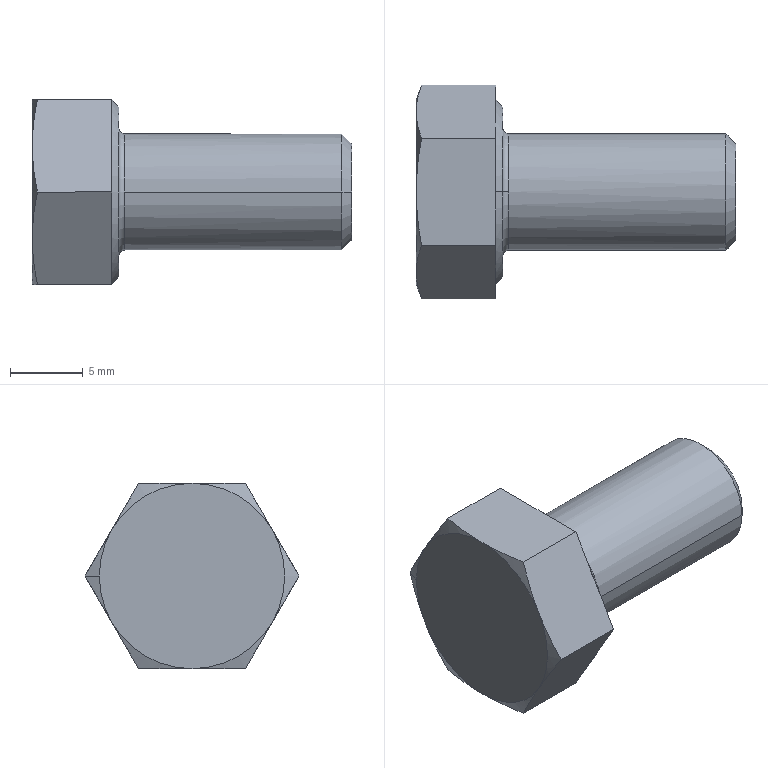Part | NX | features BREP 1 | 1 solid | 30 faces | box 21.95 x 14.699 x 12.73 mm | volume 1621 mm3 | plane 15 | cone 11 | torus 2 | cylinder 2 | commonest cylinder face diameters 8 x2
STEP:
#1=CARTESIAN_POINT('',(5.45,0.,-6.365));
#2=VERTEX_POINT('',#1);
#3=CARTESIAN_POINT('',(5.95,0.,-5.815));
#4=VERTEX_POINT('',#3);
#5=CARTESIAN_POINT('',(5.95,0.,-5.815));
#6=DIRECTION('',(-0.6727,0.,-0.7399));
#7=VECTOR('',#6,1000.);
#8=LINE('',#5,#7);
#9=EDGE_CURVE('',#2,#4,#8,.F.);
#10=ORIENTED_EDGE('',*,*,#9,.T.);
#11=CARTESIAN_POINT('',(5.95,0.,5.815));
#12=VERTEX_POINT('',#11);
#13=CARTESIAN_POINT('',(5.95,0.,0.));
#14=DIRECTION('',(-1.,0.,0.));
#15=DIRECTION('',(0.,0.,1.));
#16=AXIS2_PLACEMENT_3D('',#13,#14,#15);
#17=CIRCLE('',#16,5.815);
#18=EDGE_CURVE('',#4,#12,#17,.T.);
#19=ORIENTED_EDGE('',*,*,#18,.T.);
#20=CARTESIAN_POINT('',(5.45,0.,6.365));
#21=VERTEX_POINT('',#20);
#22=CARTESIAN_POINT('',(5.95,0.,5.815));
#23=DIRECTION('',(-0.6727,0.,0.7399));
#24=VECTOR('',#23,1000.);
#25=LINE('',#22,#24);
#26=EDGE_CURVE('',#21,#12,#25,.F.);
#27=ORIENTED_EDGE('',*,*,#26,.F.);
#28=CARTESIAN_POINT('',(5.45,-5.512,3.183));
#29=VERTEX_POINT('',#28);
#30=CARTESIAN_POINT('',(5.45,0.,0.));
#31=DIRECTION('',(-1.,0.,0.));
#32=DIRECTION('',(0.,0.,1.));
#33=AXIS2_PLACEMENT_3D('',#30,#31,#32);
#34=CIRCLE('',#33,6.365);
#35=EDGE_CURVE('',#29,#21,#34,.T.);
#36=ORIENTED_EDGE('',*,*,#35,.F.);
#37=CARTESIAN_POINT('',(5.45,-5.512,-3.183));
#38=VERTEX_POINT('',#37);
#39=CARTESIAN_POINT('',(5.45,0.,0.));
#40=DIRECTION('',(-1.,0.,0.));
#41=DIRECTION('',(0.,0.,1.));
#42=AXIS2_PLACEMENT_3D('',#39,#40,#41);
#43=CIRCLE('',#42,6.365);
#44=EDGE_CURVE('',#38,#29,#43,.T.);
#45=ORIENTED_EDGE('',*,*,#44,.F.);
#46=CARTESIAN_POINT('',(5.45,0.,0.));
#47=DIRECTION('',(-1.,0.,0.));
#48=DIRECTION('',(0.,0.,1.));
#49=AXIS2_PLACEMENT_3D('',#46,#47,#48);
#50=CIRCLE('',#49,6.365);
#51=EDGE_CURVE('',#2,#38,#50,.T.);
#52=ORIENTED_EDGE('',*,*,#51,.F.);
#53=EDGE_LOOP('',(#10,#19,#27,#36,#45,#52));
#54=FACE_BOUND('',#53,.T.);
#55=CARTESIAN_POINT('',(5.95,0.,0.));
#56=DIRECTION('',(-1.,0.,0.));
#57=DIRECTION('',(0.,0.,-1.));
#58=AXIS2_PLACEMENT_3D('',#55,#56,#57);
#59=CONICAL_SURFACE('',#58,5.815,0.833);
#60=ADVANCED_FACE('',(#54),#59,.T.);
#61=CARTESIAN_POINT('',(5.95,0.,4.4));
#62=VERTEX_POINT('',#61);
#63=CARTESIAN_POINT('',(5.95,0.,-4.4));
#64=VERTEX_POINT('',#63);
#65=CARTESIAN_POINT('',(5.95,0.,0.));
#66=DIRECTION('',(-1.,0.,0.));
#67=DIRECTION('',(0.,0.,1.));
#68=AXIS2_PLACEMENT_3D('',#65,#66,#67);
#69=CIRCLE('',#68,4.4);
#70=EDGE_CURVE('',#62,#64,#69,.T.);
#71=ORIENTED_EDGE('',*,*,#70,.T.);
#72=CARTESIAN_POINT('',(5.95,0.,0.));
#73=DIRECTION('',(-1.,0.,0.));
#74=DIRECTION('',(0.,0.,1.));
#75=AXIS2_PLACEMENT_3D('',#72,#73,#74);
#76=CIRCLE('',#75,4.4);
#77=EDGE_CURVE('',#64,#62,#76,.T.);
#78=ORIENTED_EDGE('',*,*,#77,.T.);
#79=EDGE_LOOP('',(#71,#78));
#80=FACE_BOUND('',#79,.T.);
#81=CARTESIAN_POINT('',(5.95,0.,0.));
#82=DIRECTION('',(-1.,0.,0.));
#83=DIRECTION('',(0.,0.,1.));
#84=AXIS2_PLACEMENT_3D('',#81,#82,#83);
#85=CIRCLE('',#84,5.815);
#86=EDGE_CURVE('',#12,#4,#85,.T.);
#87=ORIENTED_EDGE('',*,*,#86,.F.);
#88=ORIENTED_EDGE('',*,*,#18,.F.);
#89=EDGE_LOOP('',(#87,#88));
#90=FACE_BOUND('',#89,.T.);
#91=CARTESIAN_POINT('',(5.95,0.,0.));
#92=DIRECTION('',(-1.,0.,0.));
#93=DIRECTION('',(0.,0.,-1.));
#94=AXIS2_PLACEMENT_3D('',#91,#92,#93);
#95=PLANE('',#94);
#96=ADVANCED_FACE('',(#80,#90),#95,.F.);
#97=CARTESIAN_POINT('',(5.45,-3.675,6.365));
#98=VERTEX_POINT('',#97);
#99=CARTESIAN_POINT('',(5.45,-3.675,6.365));
#100=DIRECTION('',(0.,-0.5,-0.866));
#101=VECTOR('',#100,1000.);
#102=LINE('',#99,#101);
#103=EDGE_CURVE('',#98,#29,#102,.T.);
#104=ORIENTED_EDGE('',*,*,#103,.T.);
#105=ORIENTED_EDGE('',*,*,#35,.T.);
#106=CARTESIAN_POINT('',(5.45,3.675,6.365));
#107=DIRECTION('',(0.,-1.,0.));
#108=VECTOR('',#107,1000.);
#109=LINE('',#106,#108);
#110=EDGE_CURVE('',#21,#98,#109,.T.);
#111=ORIENTED_EDGE('',*,*,#110,.T.);
#112=EDGE_LOOP('',(#104,#105,#111));
#113=FACE_BOUND('',#112,.T.);
#114=CARTESIAN_POINT('',(5.45,0.,12.73));
#115=DIRECTION('',(-1.,0.,0.));
#116=DIRECTION('',(0.,0.,-1.));
#117=AXIS2_PLACEMENT_3D('',#114,#115,#116);
#118=PLANE('',#117);
#119=ADVANCED_FACE('',(#113),#118,.F.);
#120=ORIENTED_EDGE('',*,*,#86,.T.);
#121=ORIENTED_EDGE('',*,*,#9,.F.);
#122=CARTESIAN_POINT('',(5.45,5.512,-3.183));
#123=VERTEX_POINT('',#122);
#124=CARTESIAN_POINT('',(5.45,0.,0.));
#125=DIRECTION('',(-1.,0.,0.));
#126=DIRECTION('',(0.,0.,1.));
#127=AXIS2_PLACEMENT_3D('',#124,#125,#126);
#128=CIRCLE('',#127,6.365);
#129=EDGE_CURVE('',#123,#2,#128,.T.);
#130=ORIENTED_EDGE('',*,*,#129,.F.);
#131=CARTESIAN_POINT('',(5.45,5.512,3.183));
#132=VERTEX_POINT('',#131);
#133=CARTESIAN_POINT('',(5.45,0.,0.));
#134=DIRECTION('',(-1.,0.,0.));
#135=DIRECTION('',(0.,0.,1.));
#136=AXIS2_PLACEMENT_3D('',#133,#134,#135);
#137=CIRCLE('',#136,6.365);
#138=EDGE_CURVE('',#132,#123,#137,.T.);
#139=ORIENTED_EDGE('',*,*,#138,.F.);
#140=CARTESIAN_POINT('',(5.45,0.,0.));
#141=DIRECTION('',(-1.,0.,0.));
#142=DIRECTION('',(0.,0.,1.));
#143=AXIS2_PLACEMENT_3D('',#140,#141,#142);
#144=CIRCLE('',#143,6.365);
#145=EDGE_CURVE('',#21,#132,#144,.T.);
#146=ORIENTED_EDGE('',*,*,#145,.F.);
#147=ORIENTED_EDGE('',*,*,#26,.T.);
#148=EDGE_LOOP('',(#120,#121,#130,#139,#146,#147));
#149=FACE_BOUND('',#148,.T.);
#150=CARTESIAN_POINT('',(5.95,0.,0.));
#151=DIRECTION('',(-1.,0.,0.));
#152=DIRECTION('',(0.,0.,-1.));
#153=AXIS2_PLACEMENT_3D('',#150,#151,#152);
#154=CONICAL_SURFACE('',#153,5.815,0.833);
#155=ADVANCED_FACE('',(#149),#154,.T.);
#156=CARTESIAN_POINT('',(5.45,-3.675,-6.365));
#157=VERTEX_POINT('',#156);
#158=CARTESIAN_POINT('',(5.45,-3.675,-6.365));
#159=DIRECTION('',(0.,1.,0.));
#160=VECTOR('',#159,1000.);
#161=LINE('',#158,#160);
#162=EDGE_CURVE('',#157,#2,#161,.T.);
#163=ORIENTED_EDGE('',*,*,#162,.T.);
#164=ORIENTED_EDGE('',*,*,#51,.T.);
#165=CARTESIAN_POINT('',(5.45,-7.35,0.));
#166=DIRECTION('',(0.,0.5,-0.866));
#167=VECTOR('',#166,1000.);
#168=LINE('',#165,#167);
#169=EDGE_CURVE('',#38,#157,#168,.T.);
#170=ORIENTED_EDGE('',*,*,#169,.T.);
#171=EDGE_LOOP('',(#163,#164,#170));
#172=FACE_BOUND('',#171,.T.);
#173=CARTESIAN_POINT('',(5.45,0.,12.73));
#174=DIRECTION('',(-1.,0.,0.));
#175=DIRECTION('',(0.,0.,-1.));
#176=AXIS2_PLACEMENT_3D('',#173,#174,#175);
#177=PLANE('',#176);
#178=ADVANCED_FACE('',(#172),#177,.F.);
#179=CARTESIAN_POINT('',(5.45,-7.35,0.));
#180=VERTEX_POINT('',#179);
#181=CARTESIAN_POINT('',(5.45,-7.35,0.));
#182=DIRECTION('',(0.,0.5,-0.866));
#183=VECTOR('',#182,1000.);
#184=LINE('',#181,#183);
#185=EDGE_CURVE('',#180,#38,#184,.T.);
#186=ORIENTED_EDGE('',*,*,#185,.T.);
#187=ORIENTED_EDGE('',*,*,#44,.T.);
#188=CARTESIAN_POINT('',(5.45,-3.675,6.365));
#189=DIRECTION('',(0.,-0.5,-0.866));
#190=VECTOR('',#189,1000.);
#191=LINE('',#188,#190);
#192=EDGE_CURVE('',#29,#180,#191,.T.);
#193=ORIENTED_EDGE('',*,*,#192,.T.);
#194=EDGE_LOOP('',(#186,#187,#193));
#195=FACE_BOUND('',#194,.T.);
#196=CARTESIAN_POINT('',(5.45,0.,12.73));
#197=DIRECTION('',(-1.,0.,0.));
#198=DIRECTION('',(0.,0.,-1.));
#199=AXIS2_PLACEMENT_3D('',#196,#197,#198);
#200=PLANE('',#199);
#201=ADVANCED_FACE('',(#195),#200,.F.);
#202=ORIENTED_EDGE('',*,*,#77,.F.);
#203=CARTESIAN_POINT('',(6.35,0.,-4.));
#204=VERTEX_POINT('',#203);
#205=CARTESIAN_POINT('',(6.35,0.,-4.4));
#206=DIRECTION('',(0.,1.,0.));
#207=DIRECTION('',(0.,0.,1.));
#208=AXIS2_PLACEMENT_3D('',#205,#206,#207);
#209=CIRCLE('',#208,0.4);
#210=EDGE_CURVE('',#64,#204,#209,.T.);
#211=ORIENTED_EDGE('',*,*,#210,.T.);
#212=CARTESIAN_POINT('',(6.35,-4.,0.));
#213=VERTEX_POINT('',#212);
#214=CARTESIAN_POINT('',(6.35,0.,0.));
#215=DIRECTION('',(1.,0.,0.));
#216=DIRECTION('',(0.,0.,1.));
#217=AXIS2_PLACEMENT_3D('',#214,#215,#216);
#218=CIRCLE('',#217,4.);
#219=EDGE_CURVE('',#213,#204,#218,.T.);
#220=ORIENTED_EDGE('',*,*,#219,.F.);
#221=CARTESIAN_POINT('',(6.35,0.,4.));
#222=VERTEX_POINT('',#221);
#223=CARTESIAN_POINT('',(6.35,0.,0.));
#224=DIRECTION('',(1.,0.,0.));
#225=DIRECTION('',(0.,0.,1.));
#226=AXIS2_PLACEMENT_3D('',#223,#224,#225);
#227=CIRCLE('',#226,4.);
#228=EDGE_CURVE('',#222,#213,#227,.T.);
#229=ORIENTED_EDGE('',*,*,#228,.F.);
#230=CARTESIAN_POINT('',(6.35,0.,4.4));
#231=DIRECTION('',(0.,-1.,0.));
#232=DIRECTION('',(0.,0.,-1.));
#233=AXIS2_PLACEMENT_3D('',#230,#231,#232);
#234=CIRCLE('',#233,0.4);
#235=EDGE_CURVE('',#62,#222,#234,.T.);
#236=ORIENTED_EDGE('',*,*,#235,.F.);
#237=EDGE_LOOP('',(#202,#211,#220,#229,#236));
#238=FACE_BOUND('',#237,.T.);
#239=CARTESIAN_POINT('',(6.35,0.,0.));
#240=DIRECTION('',(-1.,0.,0.));
#241=DIRECTION('',(0.,0.,-1.));
#242=AXIS2_PLACEMENT_3D('',#239,#240,#241);
#243=TOROIDAL_SURFACE('',#242,4.4,0.4);
#244=ADVANCED_FACE('',(#238),#243,.F.);
#245=ORIENTED_EDGE('',*,*,#210,.F.);
#246=ORIENTED_EDGE('',*,*,#70,.F.);
#247=ORIENTED_EDGE('',*,*,#235,.T.);
#248=CARTESIAN_POINT('',(6.35,4.,0.));
#249=VERTEX_POINT('',#248);
#250=CARTESIAN_POINT('',(6.35,0.,0.));
#251=DIRECTION('',(1.,0.,0.));
#252=DIRECTION('',(0.,0.,1.));
#253=AXIS2_PLACEMENT_3D('',#250,#251,#252);
#254=CIRCLE('',#253,4.);
#255=EDGE_CURVE('',#249,#222,#254,.T.);
#256=ORIENTED_EDGE('',*,*,#255,.F.);
#257=CARTESIAN_POINT('',(6.35,0.,0.));
#258=DIRECTION('',(1.,0.,0.));
#259=DIRECTION('',(0.,0.,1.));
#260=AXIS2_PLACEMENT_3D('',#257,#258,#259);
#261=CIRCLE('',#260,4.);
#262=EDGE_CURVE('',#204,#249,#261,.T.);
#263=ORIENTED_EDGE('',*,*,#262,.F.);
#264=EDGE_LOOP('',(#245,#246,#247,#256,#263));
#265=FACE_BOUND('',#264,.T.);
#266=CARTESIAN_POINT('',(6.35,0.,0.));
#267=DIRECTION('',(-1.,0.,0.));
#268=DIRECTION('',(0.,0.,-1.));
#269=AXIS2_PLACEMENT_3D('',#266,#267,#268);
#270=TOROIDAL_SURFACE('',#269,4.4,0.4);
#271=ADVANCED_FACE('',(#265),#270,.F.);
#272=CARTESIAN_POINT('',(0.3584,-3.675,6.365));
#273=VERTEX_POINT('',#272);
#274=CARTESIAN_POINT('',(0.,0.,6.365));
#275=VERTEX_POINT('',#274);
#276=CARTESIAN_POINT('',(0.3584,-3.675,6.365));
#277=CARTESIAN_POINT('',(0.1373,-2.46,6.365));
#278=CARTESIAN_POINT('',(0.,-1.237,6.365));
#279=CARTESIAN_POINT('',(0.,0.,6.365));
#280=B_SPLINE_CURVE_WITH_KNOTS('',3,(#276,#277,#278,#279),.UNSPECIFIED.,.F.,.F.,(4,4),(0.,0.003692),.UNSPECIFIED.);
#281=EDGE_CURVE('',#273,#275,#280,.T.);
#282=ORIENTED_EDGE('',*,*,#281,.F.);
#283=CARTESIAN_POINT('',(5.45,-3.675,6.365));
#284=DIRECTION('',(-1.,0.,0.));
#285=VECTOR('',#284,1000.);
#286=LINE('',#283,#285);
#287=EDGE_CURVE('',#98,#273,#286,.T.);
#288=ORIENTED_EDGE('',*,*,#287,.F.);
#289=ORIENTED_EDGE('',*,*,#110,.F.);
#290=CARTESIAN_POINT('',(5.45,3.675,6.365));
#291=VERTEX_POINT('',#290);
#292=CARTESIAN_POINT('',(5.45,3.675,6.365));
#293=DIRECTION('',(0.,-1.,0.));
#294=VECTOR('',#293,1000.);
#295=LINE('',#292,#294);
#296=EDGE_CURVE('',#291,#21,#295,.T.);
#297=ORIENTED_EDGE('',*,*,#296,.F.);
#298=CARTESIAN_POINT('',(0.3584,3.675,6.365));
#299=VERTEX_POINT('',#298);
#300=CARTESIAN_POINT('',(5.45,3.675,6.365));
#301=DIRECTION('',(-1.,0.,0.));
#302=VECTOR('',#301,1000.);
#303=LINE('',#300,#302);
#304=EDGE_CURVE('',#291,#299,#303,.T.);
#305=ORIENTED_EDGE('',*,*,#304,.T.);
#306=CARTESIAN_POINT('',(0.,0.,6.365));
#307=CARTESIAN_POINT('',(0.,1.237,6.365));
#308=CARTESIAN_POINT('',(0.1373,2.46,6.365));
#309=CARTESIAN_POINT('',(0.3584,3.675,6.365));
#310=B_SPLINE_CURVE_WITH_KNOTS('',3,(#306,#307,#308,#309),.UNSPECIFIED.,.F.,.F.,(4,4),(0.,0.003692),.UNSPECIFIED.);
#311=EDGE_CURVE('',#275,#299,#310,.T.);
#312=ORIENTED_EDGE('',*,*,#311,.F.);
#313=EDGE_LOOP('',(#282,#288,#289,#297,#305,#312));
#314=FACE_BOUND('',#313,.T.);
#315=CARTESIAN_POINT('',(5.45,3.675,6.365));
#316=DIRECTION('',(0.,0.,-1.));
#317=DIRECTION('',(1.,0.,0.));
#318=AXIS2_PLACEMENT_3D('',#315,#316,#317);
#319=PLANE('',#318);
#320=ADVANCED_FACE('',(#314),#319,.F.);
#321=CARTESIAN_POINT('',(0.3584,-7.35,0.));
#322=VERTEX_POINT('',#321);
#323=CARTESIAN_POINT('',(0.,-5.512,3.183));
#324=VERTEX_POINT('',#323);
#325=CARTESIAN_POINT('',(0.3584,-7.35,0.));
#326=CARTESIAN_POINT('',(0.1373,-6.742,1.052));
#327=CARTESIAN_POINT('',(0.,-6.131,2.112));
#328=CARTESIAN_POINT('',(0.,-5.512,3.183));
#329=B_SPLINE_CURVE_WITH_KNOTS('',3,(#325,#326,#327,#328),.UNSPECIFIED.,.F.,.F.,(4,4),(0.,0.003692),.UNSPECIFIED.);
#330=EDGE_CURVE('',#322,#324,#329,.T.);
#331=ORIENTED_EDGE('',*,*,#330,.F.);
#332=CARTESIAN_POINT('',(5.45,-7.35,0.));
#333=DIRECTION('',(-1.,0.,0.));
#334=VECTOR('',#333,1000.);
#335=LINE('',#332,#334);
#336=EDGE_CURVE('',#180,#322,#335,.T.);
#337=ORIENTED_EDGE('',*,*,#336,.F.);
#338=ORIENTED_EDGE('',*,*,#192,.F.);
#339=ORIENTED_EDGE('',*,*,#103,.F.);
#340=ORIENTED_EDGE('',*,*,#287,.T.);
#341=CARTESIAN_POINT('',(0.,-5.512,3.183));
#342=CARTESIAN_POINT('',(0.,-4.894,4.253));
#343=CARTESIAN_POINT('',(0.1373,-4.282,5.313));
#344=CARTESIAN_POINT('',(0.3584,-3.675,6.365));
#345=B_SPLINE_CURVE_WITH_KNOTS('',3,(#341,#342,#343,#344),.UNSPECIFIED.,.F.,.F.,(4,4),(0.,0.003692),.UNSPECIFIED.);
#346=EDGE_CURVE('',#324,#273,#345,.T.);
#347=ORIENTED_EDGE('',*,*,#346,.F.);
#348=EDGE_LOOP('',(#331,#337,#338,#339,#340,#347));
#349=FACE_BOUND('',#348,.T.);
#350=CARTESIAN_POINT('',(5.45,-3.675,6.365));
#351=DIRECTION('',(0.,0.866,-0.5));
#352=DIRECTION('',(0.,-0.5,-0.866));
#353=AXIS2_PLACEMENT_3D('',#350,#351,#352);
#354=PLANE('',#353);
#355=ADVANCED_FACE('',(#349),#354,.F.);
#356=CARTESIAN_POINT('',(5.45,7.35,0.));
#357=VERTEX_POINT('',#356);
#358=CARTESIAN_POINT('',(5.45,7.35,0.));
#359=DIRECTION('',(0.,-0.5,0.866));
#360=VECTOR('',#359,1000.);
#361=LINE('',#358,#360);
#362=EDGE_CURVE('',#357,#132,#361,.T.);
#363=ORIENTED_EDGE('',*,*,#362,.T.);
#364=ORIENTED_EDGE('',*,*,#138,.T.);
#365=CARTESIAN_POINT('',(5.45,3.675,-6.365));
#366=DIRECTION('',(0.,0.5,0.866));
#367=VECTOR('',#366,1000.);
#368=LINE('',#365,#367);
#369=EDGE_CURVE('',#123,#357,#368,.T.);
#370=ORIENTED_EDGE('',*,*,#369,.T.);
#371=EDGE_LOOP('',(#363,#364,#370));
#372=FACE_BOUND('',#371,.T.);
#373=CARTESIAN_POINT('',(5.45,0.,12.73));
#374=DIRECTION('',(-1.,0.,0.));
#375=DIRECTION('',(0.,0.,-1.));
#376=AXIS2_PLACEMENT_3D('',#373,#374,#375);
#377=PLANE('',#376);
#378=ADVANCED_FACE('',(#372),#377,.F.);
#379=CARTESIAN_POINT('',(5.45,3.675,-6.365));
#380=VERTEX_POINT('',#379);
#381=CARTESIAN_POINT('',(5.45,3.675,-6.365));
#382=DIRECTION('',(0.,0.5,0.866));
#383=VECTOR('',#382,1000.);
#384=LINE('',#381,#383);
#385=EDGE_CURVE('',#380,#123,#384,.T.);
#386=ORIENTED_EDGE('',*,*,#385,.T.);
#387=ORIENTED_EDGE('',*,*,#129,.T.);
#388=CARTESIAN_POINT('',(5.45,-3.675,-6.365));
#389=DIRECTION('',(0.,1.,0.));
#390=VECTOR('',#389,1000.);
#391=LINE('',#388,#390);
#392=EDGE_CURVE('',#2,#380,#391,.T.);
#393=ORIENTED_EDGE('',*,*,#392,.T.);
#394=EDGE_LOOP('',(#386,#387,#393));
#395=FACE_BOUND('',#394,.T.);
#396=CARTESIAN_POINT('',(5.45,0.,12.73));
#397=DIRECTION('',(-1.,0.,0.));
#398=DIRECTION('',(0.,0.,-1.));
#399=AXIS2_PLACEMENT_3D('',#396,#397,#398);
#400=PLANE('',#399);
#401=ADVANCED_FACE('',(#395),#400,.F.);
#402=ORIENTED_EDGE('',*,*,#296,.T.);
#403=ORIENTED_EDGE('',*,*,#145,.T.);
#404=CARTESIAN_POINT('',(5.45,7.35,0.));
#405=DIRECTION('',(0.,-0.5,0.866));
#406=VECTOR('',#405,1000.);
#407=LINE('',#404,#406);
#408=EDGE_CURVE('',#132,#291,#407,.T.);
#409=ORIENTED_EDGE('',*,*,#408,.T.);
#410=EDGE_LOOP('',(#402,#403,#409));
#411=FACE_BOUND('',#410,.T.);
#412=CARTESIAN_POINT('',(5.45,0.,12.73));
#413=DIRECTION('',(-1.,0.,0.));
#414=DIRECTION('',(0.,0.,-1.));
#415=AXIS2_PLACEMENT_3D('',#412,#413,#414);
#416=PLANE('',#415);
#417=ADVANCED_FACE('',(#411),#416,.F.);
#418=CARTESIAN_POINT('',(0.3584,3.675,-6.365));
#419=VERTEX_POINT('',#418);
#420=CARTESIAN_POINT('',(0.,0.,-6.365));
#421=VERTEX_POINT('',#420);
#422=CARTESIAN_POINT('',(0.3584,3.675,-6.365));
#423=CARTESIAN_POINT('',(0.1373,2.46,-6.365));
#424=CARTESIAN_POINT('',(0.,1.237,-6.365));
#425=CARTESIAN_POINT('',(0.,0.,-6.365));
#426=B_SPLINE_CURVE_WITH_KNOTS('',3,(#422,#423,#424,#425),.UNSPECIFIED.,.F.,.F.,(4,4),(0.,0.003692),.UNSPECIFIED.);
#427=EDGE_CURVE('',#419,#421,#426,.T.);
#428=ORIENTED_EDGE('',*,*,#427,.F.);
#429=CARTESIAN_POINT('',(5.45,3.675,-6.365));
#430=DIRECTION('',(-1.,0.,0.));
#431=VECTOR('',#430,1000.);
#432=LINE('',#429,#431);
#433=EDGE_CURVE('',#380,#419,#432,.T.);
#434=ORIENTED_EDGE('',*,*,#433,.F.);
#435=ORIENTED_EDGE('',*,*,#392,.F.);
#436=ORIENTED_EDGE('',*,*,#162,.F.);
#437=CARTESIAN_POINT('',(0.3584,-3.675,-6.365));
#438=VERTEX_POINT('',#437);
#439=CARTESIAN_POINT('',(5.45,-3.675,-6.365));
#440=DIRECTION('',(-1.,0.,0.));
#441=VECTOR('',#440,1000.);
#442=LINE('',#439,#441);
#443=EDGE_CURVE('',#157,#438,#442,.T.);
#444=ORIENTED_EDGE('',*,*,#443,.T.);
#445=CARTESIAN_POINT('',(0.,0.,-6.365));
#446=CARTESIAN_POINT('',(0.,-1.237,-6.365));
#447=CARTESIAN_POINT('',(0.1373,-2.46,-6.365));
#448=CARTESIAN_POINT('',(0.3584,-3.675,-6.365));
#449=B_SPLINE_CURVE_WITH_KNOTS('',3,(#445,#446,#447,#448),.UNSPECIFIED.,.F.,.F.,(4,4),(0.,0.003692),.UNSPECIFIED.);
#450=EDGE_CURVE('',#421,#438,#449,.T.);
#451=ORIENTED_EDGE('',*,*,#450,.F.);
#452=EDGE_LOOP('',(#428,#434,#435,#436,#444,#451));
#453=FACE_BOUND('',#452,.T.);
#454=CARTESIAN_POINT('',(5.45,-3.675,-6.365));
#455=DIRECTION('',(0.,0.,1.));
#456=DIRECTION('',(0.,1.,0.));
#457=AXIS2_PLACEMENT_3D('',#454,#455,#456);
#458=PLANE('',#457);
#459=ADVANCED_FACE('',(#453),#458,.F.);
#460=CARTESIAN_POINT('',(0.,-5.512,-3.183));
#461=VERTEX_POINT('',#460);
#462=CARTESIAN_POINT('',(0.3584,-3.675,-6.365));
#463=CARTESIAN_POINT('',(0.1373,-4.282,-5.313));
#464=CARTESIAN_POINT('',(0.,-4.894,-4.253));
#465=CARTESIAN_POINT('',(0.,-5.512,-3.183));
#466=B_SPLINE_CURVE_WITH_KNOTS('',3,(#462,#463,#464,#465),.UNSPECIFIED.,.F.,.F.,(4,4),(0.,0.003692),.UNSPECIFIED.);
#467=EDGE_CURVE('',#438,#461,#466,.T.);
#468=ORIENTED_EDGE('',*,*,#467,.F.);
#469=ORIENTED_EDGE('',*,*,#443,.F.);
#470=ORIENTED_EDGE('',*,*,#169,.F.);
#471=ORIENTED_EDGE('',*,*,#185,.F.);
#472=ORIENTED_EDGE('',*,*,#336,.T.);
#473=CARTESIAN_POINT('',(0.,-5.512,-3.183));
#474=CARTESIAN_POINT('',(0.,-6.131,-2.112));
#475=CARTESIAN_POINT('',(0.1373,-6.742,-1.052));
#476=CARTESIAN_POINT('',(0.3584,-7.35,0.));
#477=B_SPLINE_CURVE_WITH_KNOTS('',3,(#473,#474,#475,#476),.UNSPECIFIED.,.F.,.F.,(4,4),(0.,0.003692),.UNSPECIFIED.);
#478=EDGE_CURVE('',#461,#322,#477,.T.);
#479=ORIENTED_EDGE('',*,*,#478,.F.);
#480=EDGE_LOOP('',(#468,#469,#470,#471,#472,#479));
#481=FACE_BOUND('',#480,.T.);
#482=CARTESIAN_POINT('',(5.45,-7.35,0.));
#483=DIRECTION('',(0.,0.866,0.5));
#484=DIRECTION('',(0.,0.5,-0.866));
#485=AXIS2_PLACEMENT_3D('',#482,#483,#484);
#486=PLANE('',#485);
#487=ADVANCED_FACE('',(#481),#486,.F.);
#488=CARTESIAN_POINT('',(21.273,4.,0.));
#489=VERTEX_POINT('',#488);
#490=CARTESIAN_POINT('',(21.95,4.,0.));
#491=DIRECTION('',(-1.,0.,0.));
#492=VECTOR('',#491,1000.);
#493=LINE('',#490,#492);
#494=EDGE_CURVE('',#489,#249,#493,.T.);
#495=ORIENTED_EDGE('',*,*,#494,.F.);
#496=CARTESIAN_POINT('',(21.273,-4.,0.));
#497=VERTEX_POINT('',#496);
#498=CARTESIAN_POINT('',(21.273,0.,0.));
#499=DIRECTION('',(-1.,0.,0.));
#500=DIRECTION('',(0.,1.,0.));
#501=AXIS2_PLACEMENT_3D('',#498,#499,#500);
#502=CIRCLE('',#501,4.);
#503=EDGE_CURVE('',#489,#497,#502,.T.);
#504=ORIENTED_EDGE('',*,*,#503,.T.);
#505=CARTESIAN_POINT('',(21.95,-4.,0.));
#506=DIRECTION('',(-1.,0.,0.));
#507=VECTOR('',#506,1000.);
#508=LINE('',#505,#507);
#509=EDGE_CURVE('',#497,#213,#508,.T.);
#510=ORIENTED_EDGE('',*,*,#509,.T.);
#511=ORIENTED_EDGE('',*,*,#219,.T.);
#512=ORIENTED_EDGE('',*,*,#262,.T.);
#513=EDGE_LOOP('',(#495,#504,#510,#511,#512));
#514=FACE_BOUND('',#513,.T.);
#515=CARTESIAN_POINT('',(21.95,0.,0.));
#516=DIRECTION('',(-1.,0.,0.));
#517=DIRECTION('',(0.,1.,0.));
#518=AXIS2_PLACEMENT_3D('',#515,#516,#517);
#519=CYLINDRICAL_SURFACE('',#518,4.);
#520=ADVANCED_FACE('',(#514),#519,.T.);
#521=CARTESIAN_POINT('',(21.273,0.,0.));
#522=DIRECTION('',(-1.,0.,0.));
#523=DIRECTION('',(0.,1.,0.));
#524=AXIS2_PLACEMENT_3D('',#521,#522,#523);
#525=CIRCLE('',#524,4.);
#526=EDGE_CURVE('',#497,#489,#525,.T.);
#527=ORIENTED_EDGE('',*,*,#526,.T.);
#528=ORIENTED_EDGE('',*,*,#494,.T.);
#529=ORIENTED_EDGE('',*,*,#255,.T.);
#530=ORIENTED_EDGE('',*,*,#228,.T.);
#531=ORIENTED_EDGE('',*,*,#509,.F.);
#532=EDGE_LOOP('',(#527,#528,#529,#530,#531));
#533=FACE_BOUND('',#532,.T.);
#534=CARTESIAN_POINT('',(21.95,0.,0.));
#535=DIRECTION('',(-1.,0.,0.));
#536=DIRECTION('',(0.,1.,0.));
#537=AXIS2_PLACEMENT_3D('',#534,#535,#536);
#538=CYLINDRICAL_SURFACE('',#537,4.);
#539=ADVANCED_FACE('',(#533),#538,.T.);
#540=ORIENTED_EDGE('',*,*,#346,.T.);
#541=ORIENTED_EDGE('',*,*,#281,.T.);
#542=CARTESIAN_POINT('',(0.,0.,0.));
#543=DIRECTION('',(-1.,0.,0.));
#544=DIRECTION('',(0.,-1.,0.));
#545=AXIS2_PLACEMENT_3D('',#542,#543,#544);
#546=CIRCLE('',#545,6.365);
#547=EDGE_CURVE('',#324,#275,#546,.T.);
#548=ORIENTED_EDGE('',*,*,#547,.F.);
#549=EDGE_LOOP('',(#540,#541,#548));
#550=FACE_BOUND('',#549,.T.);
#551=CARTESIAN_POINT('',(0.,0.,0.));
#552=DIRECTION('',(1.,0.,0.));
#553=DIRECTION('',(0.,-1.,0.));
#554=AXIS2_PLACEMENT_3D('',#551,#552,#553);
#555=CONICAL_SURFACE('',#554,6.365,1.222);
#556=ADVANCED_FACE('',(#550),#555,.T.);
#557=CARTESIAN_POINT('',(0.,5.512,3.183));
#558=VERTEX_POINT('',#557);
#559=CARTESIAN_POINT('',(0.3584,3.675,6.365));
#560=CARTESIAN_POINT('',(0.1373,4.282,5.313));
#561=CARTESIAN_POINT('',(0.,4.894,4.253));
#562=CARTESIAN_POINT('',(0.,5.512,3.183));
#563=B_SPLINE_CURVE_WITH_KNOTS('',3,(#559,#560,#561,#562),.UNSPECIFIED.,.F.,.F.,(4,4),(0.,0.003692),.UNSPECIFIED.);
#564=EDGE_CURVE('',#299,#558,#563,.T.);
#565=ORIENTED_EDGE('',*,*,#564,.T.);
#566=CARTESIAN_POINT('',(0.,0.,0.));
#567=DIRECTION('',(-1.,0.,0.));
#568=DIRECTION('',(0.,0.,1.));
#569=AXIS2_PLACEMENT_3D('',#566,#567,#568);
#570=CIRCLE('',#569,6.365);
#571=EDGE_CURVE('',#275,#558,#570,.T.);
#572=ORIENTED_EDGE('',*,*,#571,.F.);
#573=ORIENTED_EDGE('',*,*,#311,.T.);
#574=EDGE_LOOP('',(#565,#572,#573));
#575=FACE_BOUND('',#574,.T.);
#576=CARTESIAN_POINT('',(0.,0.,0.));
#577=DIRECTION('',(1.,0.,0.));
#578=DIRECTION('',(0.,-1.,0.));
#579=AXIS2_PLACEMENT_3D('',#576,#577,#578);
#580=CONICAL_SURFACE('',#579,6.365,1.222);
#581=ADVANCED_FACE('',(#575),#580,.T.);
#582=ORIENTED_EDGE('',*,*,#564,.F.);
#583=ORIENTED_EDGE('',*,*,#304,.F.);
#584=ORIENTED_EDGE('',*,*,#408,.F.);
#585=ORIENTED_EDGE('',*,*,#362,.F.);
#586=CARTESIAN_POINT('',(0.3584,7.35,0.));
#587=VERTEX_POINT('',#586);
#588=CARTESIAN_POINT('',(5.45,7.35,0.));
#589=DIRECTION('',(-1.,0.,0.));
#590=VECTOR('',#589,1000.);
#591=LINE('',#588,#590);
#592=EDGE_CURVE('',#357,#587,#591,.T.);
#593=ORIENTED_EDGE('',*,*,#592,.T.);
#594=CARTESIAN_POINT('',(0.,5.512,3.183));
#595=CARTESIAN_POINT('',(0.,6.131,2.112));
#596=CARTESIAN_POINT('',(0.1373,6.742,1.052));
#597=CARTESIAN_POINT('',(0.3584,7.35,0.));
#598=B_SPLINE_CURVE_WITH_KNOTS('',3,(#594,#595,#596,#597),.UNSPECIFIED.,.F.,.F.,(4,4),(0.,0.003692),.UNSPECIFIED.);
#599=EDGE_CURVE('',#558,#587,#598,.T.);
#600=ORIENTED_EDGE('',*,*,#599,.F.);
#601=EDGE_LOOP('',(#582,#583,#584,#585,#593,#600));
#602=FACE_BOUND('',#601,.T.);
#603=CARTESIAN_POINT('',(5.45,7.35,0.));
#604=DIRECTION('',(0.,-0.866,-0.5));
#605=DIRECTION('',(0.,-0.5,0.866));
#606=AXIS2_PLACEMENT_3D('',#603,#604,#605);
#607=PLANE('',#606);
#608=ADVANCED_FACE('',(#602),#607,.F.);
#609=ORIENTED_EDGE('',*,*,#478,.T.);
#610=ORIENTED_EDGE('',*,*,#330,.T.);
#611=CARTESIAN_POINT('',(0.,0.,0.));
#612=DIRECTION('',(-1.,0.,0.));
#613=DIRECTION('',(0.,0.,1.));
#614=AXIS2_PLACEMENT_3D('',#611,#612,#613);
#615=CIRCLE('',#614,6.365);
#616=EDGE_CURVE('',#461,#324,#615,.T.);
#617=ORIENTED_EDGE('',*,*,#616,.F.);
#618=EDGE_LOOP('',(#609,#610,#617));
#619=FACE_BOUND('',#618,.T.);
#620=CARTESIAN_POINT('',(0.,0.,0.));
#621=DIRECTION('',(1.,0.,0.));
#622=DIRECTION('',(0.,-1.,0.));
#623=AXIS2_PLACEMENT_3D('',#620,#621,#622);
#624=CONICAL_SURFACE('',#623,6.365,1.222);
#625=ADVANCED_FACE('',(#619),#624,.T.);
#626=CARTESIAN_POINT('',(0.,5.512,-3.183));
#627=VERTEX_POINT('',#626);
#628=CARTESIAN_POINT('',(0.3584,7.35,0.));
#629=CARTESIAN_POINT('',(0.1373,6.742,-1.052));
#630=CARTESIAN_POINT('',(0.,6.131,-2.112));
#631=CARTESIAN_POINT('',(0.,5.512,-3.183));
#632=B_SPLINE_CURVE_WITH_KNOTS('',3,(#628,#629,#630,#631),.UNSPECIFIED.,.F.,.F.,(4,4),(0.,0.003692),.UNSPECIFIED.);
#633=EDGE_CURVE('',#587,#627,#632,.T.);
#634=ORIENTED_EDGE('',*,*,#633,.F.);
#635=ORIENTED_EDGE('',*,*,#592,.F.);
#636=ORIENTED_EDGE('',*,*,#369,.F.);
#637=ORIENTED_EDGE('',*,*,#385,.F.);
#638=ORIENTED_EDGE('',*,*,#433,.T.);
#639=CARTESIAN_POINT('',(0.,5.512,-3.183));
#640=CARTESIAN_POINT('',(0.,4.894,-4.253));
#641=CARTESIAN_POINT('',(0.1373,4.282,-5.313));
#642=CARTESIAN_POINT('',(0.3584,3.675,-6.365));
#643=B_SPLINE_CURVE_WITH_KNOTS('',3,(#639,#640,#641,#642),.UNSPECIFIED.,.F.,.F.,(4,4),(0.,0.003692),.UNSPECIFIED.);
#644=EDGE_CURVE('',#627,#419,#643,.T.);
#645=ORIENTED_EDGE('',*,*,#644,.F.);
#646=EDGE_LOOP('',(#634,#635,#636,#637,#638,#645));
#647=FACE_BOUND('',#646,.T.);
#648=CARTESIAN_POINT('',(5.45,3.675,-6.365));
#649=DIRECTION('',(0.,-0.866,0.5));
#650=DIRECTION('',(0.,0.5,0.866));
#651=AXIS2_PLACEMENT_3D('',#648,#649,#650);
#652=PLANE('',#651);
#653=ADVANCED_FACE('',(#647),#652,.F.);
#654=ORIENTED_EDGE('',*,*,#450,.T.);
#655=ORIENTED_EDGE('',*,*,#467,.T.);
#656=CARTESIAN_POINT('',(0.,0.,0.));
#657=DIRECTION('',(-1.,0.,0.));
#658=DIRECTION('',(0.,0.,1.));
#659=AXIS2_PLACEMENT_3D('',#656,#657,#658);
#660=CIRCLE('',#659,6.365);
#661=EDGE_CURVE('',#421,#461,#660,.T.);
#662=ORIENTED_EDGE('',*,*,#661,.F.);
#663=EDGE_LOOP('',(#654,#655,#662));
#664=FACE_BOUND('',#663,.T.);
#665=CARTESIAN_POINT('',(0.,0.,0.));
#666=DIRECTION('',(1.,0.,0.));
#667=DIRECTION('',(0.,-1.,0.));
#668=AXIS2_PLACEMENT_3D('',#665,#666,#667);
#669=CONICAL_SURFACE('',#668,6.365,1.222);
#670=ADVANCED_FACE('',(#664),#669,.T.);
#671=ORIENTED_EDGE('',*,*,#427,.T.);
#672=CARTESIAN_POINT('',(0.,0.,0.));
#673=DIRECTION('',(-1.,0.,0.));
#674=DIRECTION('',(0.,0.,1.));
#675=AXIS2_PLACEMENT_3D('',#672,#673,#674);
#676=CIRCLE('',#675,6.365);
#677=EDGE_CURVE('',#627,#421,#676,.T.);
#678=ORIENTED_EDGE('',*,*,#677,.F.);
#679=ORIENTED_EDGE('',*,*,#644,.T.);
#680=EDGE_LOOP('',(#671,#678,#679));
#681=FACE_BOUND('',#680,.T.);
#682=CARTESIAN_POINT('',(0.,0.,0.));
#683=DIRECTION('',(1.,0.,0.));
#684=DIRECTION('',(0.,-1.,0.));
#685=AXIS2_PLACEMENT_3D('',#682,#683,#684);
#686=CONICAL_SURFACE('',#685,6.365,1.222);
#687=ADVANCED_FACE('',(#681),#686,.T.);
#688=CARTESIAN_POINT('',(21.95,3.324,0.));
#689=VERTEX_POINT('',#688);
#690=CARTESIAN_POINT('',(21.95,3.324,0.));
#691=DIRECTION('',(-0.7071,0.7071,0.));
#692=VECTOR('',#691,1000.);
#693=LINE('',#690,#692);
#694=EDGE_CURVE('',#689,#489,#693,.T.);
#695=ORIENTED_EDGE('',*,*,#694,.F.);
#696=CARTESIAN_POINT('',(21.95,-3.324,0.));
#697=VERTEX_POINT('',#696);
#698=CARTESIAN_POINT('',(21.95,0.,0.));
#699=DIRECTION('',(1.,0.,0.));
#700=DIRECTION('',(0.,1.,0.));
#701=AXIS2_PLACEMENT_3D('',#698,#699,#700);
#702=CIRCLE('',#701,3.324);
#703=EDGE_CURVE('',#697,#689,#702,.T.);
#704=ORIENTED_EDGE('',*,*,#703,.F.);
#705=CARTESIAN_POINT('',(21.95,-3.324,0.));
#706=DIRECTION('',(-0.7071,-0.7071,0.));
#707=VECTOR('',#706,1000.);
#708=LINE('',#705,#707);
#709=EDGE_CURVE('',#697,#497,#708,.T.);
#710=ORIENTED_EDGE('',*,*,#709,.T.);
#711=ORIENTED_EDGE('',*,*,#503,.F.);
#712=EDGE_LOOP('',(#695,#704,#710,#711));
#713=FACE_BOUND('',#712,.T.);
#714=CARTESIAN_POINT('',(21.95,0.,0.));
#715=DIRECTION('',(-1.,0.,0.));
#716=DIRECTION('',(0.,1.,0.));
#717=AXIS2_PLACEMENT_3D('',#714,#715,#716);
#718=CONICAL_SURFACE('',#717,3.324,0.7854);
#719=ADVANCED_FACE('',(#713),#718,.T.);
#720=CARTESIAN_POINT('',(21.95,0.,0.));
#721=DIRECTION('',(1.,0.,0.));
#722=DIRECTION('',(0.,1.,0.));
#723=AXIS2_PLACEMENT_3D('',#720,#721,#722);
#724=CIRCLE('',#723,3.324);
#725=EDGE_CURVE('',#689,#697,#724,.T.);
#726=ORIENTED_EDGE('',*,*,#725,.F.);
#727=ORIENTED_EDGE('',*,*,#694,.T.);
#728=ORIENTED_EDGE('',*,*,#526,.F.);
#729=ORIENTED_EDGE('',*,*,#709,.F.);
#730=EDGE_LOOP('',(#726,#727,#728,#729));
#731=FACE_BOUND('',#730,.T.);
#732=CARTESIAN_POINT('',(21.95,0.,0.));
#733=DIRECTION('',(-1.,0.,0.));
#734=DIRECTION('',(0.,1.,0.));
#735=AXIS2_PLACEMENT_3D('',#732,#733,#734);
#736=CONICAL_SURFACE('',#735,3.324,0.7854);
#737=ADVANCED_FACE('',(#731),#736,.T.);
#738=ORIENTED_EDGE('',*,*,#547,.T.);
#739=ORIENTED_EDGE('',*,*,#571,.T.);
#740=CARTESIAN_POINT('',(0.,6.365,0.));
#741=VERTEX_POINT('',#740);
#742=CARTESIAN_POINT('',(0.,0.,0.));
#743=DIRECTION('',(-1.,0.,0.));
#744=DIRECTION('',(0.,0.,1.));
#745=AXIS2_PLACEMENT_3D('',#742,#743,#744);
#746=CIRCLE('',#745,6.365);
#747=EDGE_CURVE('',#558,#741,#746,.T.);
#748=ORIENTED_EDGE('',*,*,#747,.T.);
#749=CARTESIAN_POINT('',(0.,0.,0.));
#750=DIRECTION('',(-1.,0.,0.));
#751=DIRECTION('',(0.,0.,1.));
#752=AXIS2_PLACEMENT_3D('',#749,#750,#751);
#753=CIRCLE('',#752,6.365);
#754=EDGE_CURVE('',#741,#627,#753,.T.);
#755=ORIENTED_EDGE('',*,*,#754,.T.);
#756=ORIENTED_EDGE('',*,*,#677,.T.);
#757=ORIENTED_EDGE('',*,*,#661,.T.);
#758=ORIENTED_EDGE('',*,*,#616,.T.);
#759=EDGE_LOOP('',(#738,#739,#748,#755,#756,#757,#758));
#760=FACE_BOUND('',#759,.T.);
#761=CARTESIAN_POINT('',(0.,0.,12.73));
#762=DIRECTION('',(-1.,0.,0.));
#763=DIRECTION('',(0.,0.,-1.));
#764=AXIS2_PLACEMENT_3D('',#761,#762,#763);
#765=PLANE('',#764);
#766=ADVANCED_FACE('',(#760),#765,.T.);
#767=CARTESIAN_POINT('',(0.,6.365,0.));
#768=DIRECTION('',(0.342,0.9397,0.));
#769=VECTOR('',#768,1000.);
#770=LINE('',#767,#769);
#771=EDGE_CURVE('',#741,#587,#770,.T.);
#772=ORIENTED_EDGE('',*,*,#771,.F.);
#773=ORIENTED_EDGE('',*,*,#747,.F.);
#774=ORIENTED_EDGE('',*,*,#599,.T.);
#775=EDGE_LOOP('',(#772,#773,#774));
#776=FACE_BOUND('',#775,.T.);
#777=CARTESIAN_POINT('',(0.,0.,0.));
#778=DIRECTION('',(1.,0.,0.));
#779=DIRECTION('',(0.,-1.,0.));
#780=AXIS2_PLACEMENT_3D('',#777,#778,#779);
#781=CONICAL_SURFACE('',#780,6.365,1.222);
#782=ADVANCED_FACE('',(#776),#781,.T.);
#783=ORIENTED_EDGE('',*,*,#754,.F.);
#784=ORIENTED_EDGE('',*,*,#771,.T.);
#785=ORIENTED_EDGE('',*,*,#633,.T.);
#786=EDGE_LOOP('',(#783,#784,#785));
#787=FACE_BOUND('',#786,.T.);
#788=CARTESIAN_POINT('',(0.,0.,0.));
#789=DIRECTION('',(1.,0.,0.));
#790=DIRECTION('',(0.,-1.,0.));
#791=AXIS2_PLACEMENT_3D('',#788,#789,#790);
#792=CONICAL_SURFACE('',#791,6.365,1.222);
#793=ADVANCED_FACE('',(#787),#792,.T.);
#794=ORIENTED_EDGE('',*,*,#703,.T.);
#795=ORIENTED_EDGE('',*,*,#725,.T.);
#796=EDGE_LOOP('',(#794,#795));
#797=FACE_BOUND('',#796,.T.);
#798=CARTESIAN_POINT('',(21.95,0.,0.));
#799=DIRECTION('',(1.,0.,0.));
#800=DIRECTION('',(0.,-1.,0.));
#801=AXIS2_PLACEMENT_3D('',#798,#799,#800);
#802=PLANE('',#801);
#803=ADVANCED_FACE('',(#797),#802,.T.);
#804=CLOSED_SHELL('',(#60,#96,#119,#155,#178,#201,#244,#271,#320,#355,#378,#401,#417,#459,#487,#520,#539,#556,#581,#608,#625,#653,#670,#687,#719,#737,#766,#782,#793,#803));
#805=MANIFOLD_SOLID_BREP('',#804);
#806=(LENGTH_UNIT()NAMED_UNIT(*)SI_UNIT(.MILLI.,.METRE.));
#807=UNCERTAINTY_MEASURE_WITH_UNIT(LENGTH_MEASURE(0.0508),#806,'','');
#808=(NAMED_UNIT(*)PLANE_ANGLE_UNIT()SI_UNIT($,.RADIAN.));
#809=(NAMED_UNIT(*)SI_UNIT($,.STERADIAN.)SOLID_ANGLE_UNIT());
#810=(GEOMETRIC_REPRESENTATION_CONTEXT(3)GLOBAL_UNCERTAINTY_ASSIGNED_CONTEXT((#807))GLOBAL_UNIT_ASSIGNED_CONTEXT((#806,#808,#809))REPRESENTATION_CONTEXT('',''));
#811=ADVANCED_BREP_SHAPE_REPRESENTATION('',(#805),#810);